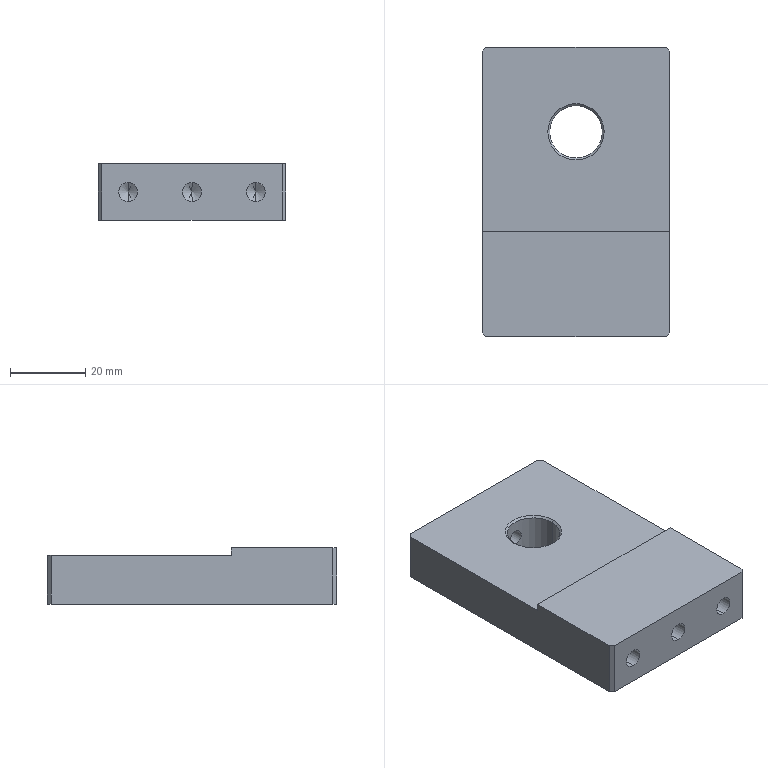Part | NX | features BREP 1 | 1 solid | 40 faces | box 50 x 77 x 15 mm | volume 49360 mm3 | cylinder 14 | cone 14 | plane 12 | commonest cylinder face diameters 5 x6 3.3 x4 4.2 x2 14 x2
STEP:
#1=CARTESIAN_POINT('',(0.,23.,-2.1));
#2=VERTEX_POINT('',#1);
#3=CARTESIAN_POINT('',(0.,23.,2.1));
#4=VERTEX_POINT('',#3);
#5=CARTESIAN_POINT('',(0.,23.,2.1));
#6=CARTESIAN_POINT('',(-0.262,23.,2.1));
#7=CARTESIAN_POINT('',(-0.7456,22.966,1.986));
#8=CARTESIAN_POINT('',(-1.093,22.916,1.805));
#9=CARTESIAN_POINT('',(-1.501,22.841,1.507));
#10=CARTESIAN_POINT('',(-1.817,22.762,1.075));
#11=CARTESIAN_POINT('',(-1.934,22.728,0.8436));
#12=CARTESIAN_POINT('',(-2.082,22.684,0.3873));
#13=CARTESIAN_POINT('',(-2.109,22.674,-0.00003847));
#14=CARTESIAN_POINT('',(-2.082,22.684,-0.3881));
#15=CARTESIAN_POINT('',(-1.934,22.728,-0.844));
#16=CARTESIAN_POINT('',(-1.817,22.762,-1.075));
#17=CARTESIAN_POINT('',(-1.5,22.842,-1.508));
#18=CARTESIAN_POINT('',(-1.092,22.916,-1.805));
#19=CARTESIAN_POINT('',(-0.7431,22.967,-1.987));
#20=CARTESIAN_POINT('',(-0.2615,23.,-2.1));
#21=CARTESIAN_POINT('',(0.,23.,-2.1));
#22=B_SPLINE_CURVE_WITH_KNOTS('',3,(#5,#6,#7,#8,#9,#10,#11,#12,#13,#14,#15,#16,#17,#18,#19,#20,#21),.UNSPECIFIED.,.F.,.F.,(4,1,1,1,1,1,1,1,1,1,1,1,1,1,4),(0.,0.125,0.1875,0.25,0.3125,0.375,0.4375,0.5,0.5625,0.625,0.6875,0.75,0.8125,0.875,1.),.UNSPECIFIED.);
#23=EDGE_CURVE('',#2,#4,#22,.F.);
#24=ORIENTED_EDGE('',*,*,#23,.F.);
#25=CARTESIAN_POINT('',(0.,38.5,-2.1));
#26=VERTEX_POINT('',#25);
#27=CARTESIAN_POINT('',(0.,38.5,-2.1));
#28=DIRECTION('',(0.,1.,0.));
#29=VECTOR('',#28,1000.);
#30=LINE('',#27,#29);
#31=EDGE_CURVE('',#26,#2,#30,.F.);
#32=ORIENTED_EDGE('',*,*,#31,.F.);
#33=CARTESIAN_POINT('',(0.,38.5,2.1));
#34=VERTEX_POINT('',#33);
#35=CARTESIAN_POINT('',(0.,38.5,0.));
#36=DIRECTION('',(0.,1.,0.));
#37=DIRECTION('',(0.,0.,1.));
#38=AXIS2_PLACEMENT_3D('',#35,#36,#37);
#39=CIRCLE('',#38,2.1);
#40=EDGE_CURVE('',#26,#34,#39,.T.);
#41=ORIENTED_EDGE('',*,*,#40,.T.);
#42=CARTESIAN_POINT('',(0.,38.5,2.1));
#43=DIRECTION('',(0.,1.,0.));
#44=VECTOR('',#43,1000.);
#45=LINE('',#42,#44);
#46=EDGE_CURVE('',#34,#4,#45,.F.);
#47=ORIENTED_EDGE('',*,*,#46,.T.);
#48=EDGE_LOOP('',(#24,#32,#41,#47));
#49=FACE_BOUND('',#48,.T.);
#50=CARTESIAN_POINT('',(0.,38.5,0.));
#51=DIRECTION('',(0.,1.,0.));
#52=DIRECTION('',(0.,0.,1.));
#53=AXIS2_PLACEMENT_3D('',#50,#51,#52);
#54=CYLINDRICAL_SURFACE('',#53,2.1);
#55=ADVANCED_FACE('',(#49),#54,.F.);
#56=CARTESIAN_POINT('',(-17.,27.,-1.65));
#57=VERTEX_POINT('',#56);
#58=CARTESIAN_POINT('',(-17.,27.,1.65));
#59=VERTEX_POINT('',#58);
#60=CARTESIAN_POINT('',(-17.,27.,0.));
#61=DIRECTION('',(0.,1.,0.));
#62=DIRECTION('',(0.,0.,1.));
#63=AXIS2_PLACEMENT_3D('',#60,#61,#62);
#64=CIRCLE('',#63,1.65);
#65=EDGE_CURVE('',#57,#59,#64,.T.);
#66=ORIENTED_EDGE('',*,*,#65,.F.);
#67=CARTESIAN_POINT('',(-17.,38.5,-1.65));
#68=VERTEX_POINT('',#67);
#69=CARTESIAN_POINT('',(-17.,38.5,-1.65));
#70=DIRECTION('',(0.,1.,0.));
#71=VECTOR('',#70,1000.);
#72=LINE('',#69,#71);
#73=EDGE_CURVE('',#68,#57,#72,.F.);
#74=ORIENTED_EDGE('',*,*,#73,.F.);
#75=CARTESIAN_POINT('',(-17.,38.5,1.65));
#76=VERTEX_POINT('',#75);
#77=CARTESIAN_POINT('',(-17.,38.5,0.));
#78=DIRECTION('',(0.,1.,0.));
#79=DIRECTION('',(0.,0.,1.));
#80=AXIS2_PLACEMENT_3D('',#77,#78,#79);
#81=CIRCLE('',#80,1.65);
#82=EDGE_CURVE('',#68,#76,#81,.T.);
#83=ORIENTED_EDGE('',*,*,#82,.T.);
#84=CARTESIAN_POINT('',(-17.,38.5,1.65));
#85=DIRECTION('',(0.,1.,0.));
#86=VECTOR('',#85,1000.);
#87=LINE('',#84,#86);
#88=EDGE_CURVE('',#76,#59,#87,.F.);
#89=ORIENTED_EDGE('',*,*,#88,.T.);
#90=EDGE_LOOP('',(#66,#74,#83,#89));
#91=FACE_BOUND('',#90,.T.);
#92=CARTESIAN_POINT('',(-17.,38.5,0.));
#93=DIRECTION('',(0.,1.,0.));
#94=DIRECTION('',(0.,0.,1.));
#95=AXIS2_PLACEMENT_3D('',#92,#93,#94);
#96=CYLINDRICAL_SURFACE('',#95,1.65);
#97=ADVANCED_FACE('',(#91),#96,.F.);
#98=CARTESIAN_POINT('',(-17.,26.009,0.));
#99=VERTEX_POINT('',#98);
#100=CARTESIAN_POINT('',(-17.,27.,1.65));
#101=DIRECTION('',(0.,0.515,0.8572));
#102=VECTOR('',#101,1000.);
#103=LINE('',#100,#102);
#104=EDGE_CURVE('',#59,#99,#103,.F.);
#105=ORIENTED_EDGE('',*,*,#104,.T.);
#106=CARTESIAN_POINT('',(-17.,27.,-1.65));
#107=DIRECTION('',(0.,0.515,-0.8572));
#108=VECTOR('',#107,1000.);
#109=LINE('',#106,#108);
#110=EDGE_CURVE('',#57,#99,#109,.F.);
#111=ORIENTED_EDGE('',*,*,#110,.F.);
#112=ORIENTED_EDGE('',*,*,#65,.T.);
#113=EDGE_LOOP('',(#105,#111,#112));
#114=FACE_BOUND('',#113,.T.);
#115=CARTESIAN_POINT('',(-17.,27.,0.));
#116=DIRECTION('',(0.,1.,0.));
#117=DIRECTION('',(0.,0.,1.));
#118=AXIS2_PLACEMENT_3D('',#115,#116,#117);
#119=CONICAL_SURFACE('',#118,1.65,1.03);
#120=ADVANCED_FACE('',(#114),#119,.F.);
#121=CARTESIAN_POINT('',(17.,27.,-1.65));
#122=VERTEX_POINT('',#121);
#123=CARTESIAN_POINT('',(17.,27.,1.65));
#124=VERTEX_POINT('',#123);
#125=CARTESIAN_POINT('',(17.,27.,0.));
#126=DIRECTION('',(0.,1.,0.));
#127=DIRECTION('',(0.,0.,1.));
#128=AXIS2_PLACEMENT_3D('',#125,#126,#127);
#129=CIRCLE('',#128,1.65);
#130=EDGE_CURVE('',#122,#124,#129,.T.);
#131=ORIENTED_EDGE('',*,*,#130,.F.);
#132=CARTESIAN_POINT('',(17.,38.5,-1.65));
#133=VERTEX_POINT('',#132);
#134=CARTESIAN_POINT('',(17.,38.5,-1.65));
#135=DIRECTION('',(0.,1.,0.));
#136=VECTOR('',#135,1000.);
#137=LINE('',#134,#136);
#138=EDGE_CURVE('',#133,#122,#137,.F.);
#139=ORIENTED_EDGE('',*,*,#138,.F.);
#140=CARTESIAN_POINT('',(17.,38.5,1.65));
#141=VERTEX_POINT('',#140);
#142=CARTESIAN_POINT('',(17.,38.5,0.));
#143=DIRECTION('',(0.,1.,0.));
#144=DIRECTION('',(0.,0.,1.));
#145=AXIS2_PLACEMENT_3D('',#142,#143,#144);
#146=CIRCLE('',#145,1.65);
#147=EDGE_CURVE('',#133,#141,#146,.T.);
#148=ORIENTED_EDGE('',*,*,#147,.T.);
#149=CARTESIAN_POINT('',(17.,38.5,1.65));
#150=DIRECTION('',(0.,1.,0.));
#151=VECTOR('',#150,1000.);
#152=LINE('',#149,#151);
#153=EDGE_CURVE('',#141,#124,#152,.F.);
#154=ORIENTED_EDGE('',*,*,#153,.T.);
#155=EDGE_LOOP('',(#131,#139,#148,#154));
#156=FACE_BOUND('',#155,.T.);
#157=CARTESIAN_POINT('',(17.,38.5,0.));
#158=DIRECTION('',(0.,1.,0.));
#159=DIRECTION('',(0.,0.,1.));
#160=AXIS2_PLACEMENT_3D('',#157,#158,#159);
#161=CYLINDRICAL_SURFACE('',#160,1.65);
#162=ADVANCED_FACE('',(#156),#161,.F.);
#163=CARTESIAN_POINT('',(17.,26.009,0.));
#164=VERTEX_POINT('',#163);
#165=CARTESIAN_POINT('',(17.,27.,1.65));
#166=DIRECTION('',(0.,0.515,0.8572));
#167=VECTOR('',#166,1000.);
#168=LINE('',#165,#167);
#169=EDGE_CURVE('',#124,#164,#168,.F.);
#170=ORIENTED_EDGE('',*,*,#169,.T.);
#171=CARTESIAN_POINT('',(17.,27.,-1.65));
#172=DIRECTION('',(0.,0.515,-0.8572));
#173=VECTOR('',#172,1000.);
#174=LINE('',#171,#173);
#175=EDGE_CURVE('',#122,#164,#174,.F.);
#176=ORIENTED_EDGE('',*,*,#175,.F.);
#177=ORIENTED_EDGE('',*,*,#130,.T.);
#178=EDGE_LOOP('',(#170,#176,#177));
#179=FACE_BOUND('',#178,.T.);
#180=CARTESIAN_POINT('',(17.,27.,0.));
#181=DIRECTION('',(0.,1.,0.));
#182=DIRECTION('',(0.,0.,1.));
#183=AXIS2_PLACEMENT_3D('',#180,#181,#182);
#184=CONICAL_SURFACE('',#183,1.65,1.03);
#185=ADVANCED_FACE('',(#179),#184,.F.);
#186=CARTESIAN_POINT('',(7.,16.,-7.));
#187=VERTEX_POINT('',#186);
#188=CARTESIAN_POINT('',(-7.,16.,-7.));
#189=VERTEX_POINT('',#188);
#190=CARTESIAN_POINT('',(0.,16.,-7.));
#191=DIRECTION('',(0.,0.,-1.));
#192=DIRECTION('',(-1.,0.,0.));
#193=AXIS2_PLACEMENT_3D('',#190,#191,#192);
#194=CIRCLE('',#193,7.);
#195=EDGE_CURVE('',#187,#189,#194,.T.);
#196=ORIENTED_EDGE('',*,*,#195,.F.);
#197=CARTESIAN_POINT('',(7.5,16.,-7.5));
#198=VERTEX_POINT('',#197);
#199=CARTESIAN_POINT('',(7.5,16.,-7.5));
#200=DIRECTION('',(0.7071,0.,-0.7071));
#201=VECTOR('',#200,1000.);
#202=LINE('',#199,#201);
#203=EDGE_CURVE('',#187,#198,#202,.T.);
#204=ORIENTED_EDGE('',*,*,#203,.T.);
#205=CARTESIAN_POINT('',(-7.5,16.,-7.5));
#206=VERTEX_POINT('',#205);
#207=CARTESIAN_POINT('',(0.,16.,-7.5));
#208=DIRECTION('',(0.,0.,1.));
#209=DIRECTION('',(-1.,0.,0.));
#210=AXIS2_PLACEMENT_3D('',#207,#208,#209);
#211=CIRCLE('',#210,7.5);
#212=EDGE_CURVE('',#206,#198,#211,.T.);
#213=ORIENTED_EDGE('',*,*,#212,.F.);
#214=CARTESIAN_POINT('',(-7.5,16.,-7.5));
#215=DIRECTION('',(-0.7071,0.,-0.7071));
#216=VECTOR('',#215,1000.);
#217=LINE('',#214,#216);
#218=EDGE_CURVE('',#189,#206,#217,.T.);
#219=ORIENTED_EDGE('',*,*,#218,.F.);
#220=EDGE_LOOP('',(#196,#204,#213,#219));
#221=FACE_BOUND('',#220,.T.);
#222=CARTESIAN_POINT('',(0.,16.,-7.5));
#223=DIRECTION('',(0.,0.,-1.));
#224=DIRECTION('',(-1.,0.,0.));
#225=AXIS2_PLACEMENT_3D('',#222,#223,#224);
#226=CONICAL_SURFACE('',#225,7.5,0.7854);
#227=ADVANCED_FACE('',(#221),#226,.F.);
#228=CARTESIAN_POINT('',(-7.,16.,5.));
#229=VERTEX_POINT('',#228);
#230=CARTESIAN_POINT('',(7.,16.,5.));
#231=VERTEX_POINT('',#230);
#232=CARTESIAN_POINT('',(0.,16.,5.));
#233=DIRECTION('',(0.,0.,1.));
#234=DIRECTION('',(1.,0.,0.));
#235=AXIS2_PLACEMENT_3D('',#232,#233,#234);
#236=CIRCLE('',#235,7.);
#237=EDGE_CURVE('',#229,#231,#236,.T.);
#238=ORIENTED_EDGE('',*,*,#237,.F.);
#239=CARTESIAN_POINT('',(-7.5,16.,5.5));
#240=VERTEX_POINT('',#239);
#241=CARTESIAN_POINT('',(-7.5,16.,5.5));
#242=DIRECTION('',(-0.7071,0.,0.7071));
#243=VECTOR('',#242,1000.);
#244=LINE('',#241,#243);
#245=EDGE_CURVE('',#240,#229,#244,.F.);
#246=ORIENTED_EDGE('',*,*,#245,.F.);
#247=CARTESIAN_POINT('',(7.5,16.,5.5));
#248=VERTEX_POINT('',#247);
#249=CARTESIAN_POINT('',(0.,16.,5.5));
#250=DIRECTION('',(0.,0.,-1.));
#251=DIRECTION('',(1.,0.,0.));
#252=AXIS2_PLACEMENT_3D('',#249,#250,#251);
#253=CIRCLE('',#252,7.5);
#254=EDGE_CURVE('',#248,#240,#253,.T.);
#255=ORIENTED_EDGE('',*,*,#254,.F.);
#256=CARTESIAN_POINT('',(7.5,16.,5.5));
#257=DIRECTION('',(0.7071,0.,0.7071));
#258=VECTOR('',#257,1000.);
#259=LINE('',#256,#258);
#260=EDGE_CURVE('',#248,#231,#259,.F.);
#261=ORIENTED_EDGE('',*,*,#260,.T.);
#262=EDGE_LOOP('',(#238,#246,#255,#261));
#263=FACE_BOUND('',#262,.T.);
#264=CARTESIAN_POINT('',(0.,16.,5.5));
#265=DIRECTION('',(0.,0.,1.));
#266=DIRECTION('',(1.,0.,0.));
#267=AXIS2_PLACEMENT_3D('',#264,#265,#266);
#268=CONICAL_SURFACE('',#267,7.5,0.7854);
#269=ADVANCED_FACE('',(#263),#268,.F.);
#270=CARTESIAN_POINT('',(-17.,-21.5,2.5));
#271=VERTEX_POINT('',#270);
#272=CARTESIAN_POINT('',(-17.,-21.5,-2.5));
#273=VERTEX_POINT('',#272);
#274=CARTESIAN_POINT('',(-17.,-21.5,0.));
#275=DIRECTION('',(0.,-1.,0.));
#276=DIRECTION('',(0.,0.,-1.));
#277=AXIS2_PLACEMENT_3D('',#274,#275,#276);
#278=CIRCLE('',#277,2.5);
#279=EDGE_CURVE('',#271,#273,#278,.T.);
#280=ORIENTED_EDGE('',*,*,#279,.F.);
#281=CARTESIAN_POINT('',(-17.,-38.5,2.5));
#282=VERTEX_POINT('',#281);
#283=CARTESIAN_POINT('',(-17.,-38.5,2.5));
#284=DIRECTION('',(0.,-1.,0.));
#285=VECTOR('',#284,1000.);
#286=LINE('',#283,#285);
#287=EDGE_CURVE('',#271,#282,#286,.T.);
#288=ORIENTED_EDGE('',*,*,#287,.T.);
#289=CARTESIAN_POINT('',(-17.,-38.5,-2.5));
#290=VERTEX_POINT('',#289);
#291=CARTESIAN_POINT('',(-17.,-38.5,0.));
#292=DIRECTION('',(0.,-1.,0.));
#293=DIRECTION('',(0.,0.,-1.));
#294=AXIS2_PLACEMENT_3D('',#291,#292,#293);
#295=CIRCLE('',#294,2.5);
#296=EDGE_CURVE('',#282,#290,#295,.T.);
#297=ORIENTED_EDGE('',*,*,#296,.T.);
#298=CARTESIAN_POINT('',(-17.,-38.5,-2.5));
#299=DIRECTION('',(0.,-1.,0.));
#300=VECTOR('',#299,1000.);
#301=LINE('',#298,#300);
#302=EDGE_CURVE('',#273,#290,#301,.T.);
#303=ORIENTED_EDGE('',*,*,#302,.F.);
#304=EDGE_LOOP('',(#280,#288,#297,#303));
#305=FACE_BOUND('',#304,.T.);
#306=CARTESIAN_POINT('',(-17.,-38.5,0.));
#307=DIRECTION('',(0.,-1.,0.));
#308=DIRECTION('',(0.,0.,-1.));
#309=AXIS2_PLACEMENT_3D('',#306,#307,#308);
#310=CYLINDRICAL_SURFACE('',#309,2.5);
#311=ADVANCED_FACE('',(#305),#310,.F.);
#312=CARTESIAN_POINT('',(-17.,-19.998,0.));
#313=VERTEX_POINT('',#312);
#314=CARTESIAN_POINT('',(-17.,-21.5,-2.5));
#315=DIRECTION('',(0.,-0.515,-0.8572));
#316=VECTOR('',#315,1000.);
#317=LINE('',#314,#316);
#318=EDGE_CURVE('',#313,#273,#317,.T.);
#319=ORIENTED_EDGE('',*,*,#318,.F.);
#320=CARTESIAN_POINT('',(-17.,-21.5,2.5));
#321=DIRECTION('',(0.,-0.515,0.8572));
#322=VECTOR('',#321,1000.);
#323=LINE('',#320,#322);
#324=EDGE_CURVE('',#313,#271,#323,.T.);
#325=ORIENTED_EDGE('',*,*,#324,.T.);
#326=ORIENTED_EDGE('',*,*,#279,.T.);
#327=EDGE_LOOP('',(#319,#325,#326));
#328=FACE_BOUND('',#327,.T.);
#329=CARTESIAN_POINT('',(-17.,-21.5,0.));
#330=DIRECTION('',(0.,-1.,0.));
#331=DIRECTION('',(0.,0.,-1.));
#332=AXIS2_PLACEMENT_3D('',#329,#330,#331);
#333=CONICAL_SURFACE('',#332,2.5,1.03);
#334=ADVANCED_FACE('',(#328),#333,.F.);
#335=CARTESIAN_POINT('',(0.,-21.5,2.5));
#336=VERTEX_POINT('',#335);
#337=CARTESIAN_POINT('',(0.,-21.5,-2.5));
#338=VERTEX_POINT('',#337);
#339=CARTESIAN_POINT('',(0.,-21.5,0.));
#340=DIRECTION('',(0.,-1.,0.));
#341=DIRECTION('',(0.,0.,-1.));
#342=AXIS2_PLACEMENT_3D('',#339,#340,#341);
#343=CIRCLE('',#342,2.5);
#344=EDGE_CURVE('',#336,#338,#343,.T.);
#345=ORIENTED_EDGE('',*,*,#344,.F.);
#346=CARTESIAN_POINT('',(0.,-38.5,2.5));
#347=VERTEX_POINT('',#346);
#348=CARTESIAN_POINT('',(0.,-38.5,2.5));
#349=DIRECTION('',(0.,-1.,0.));
#350=VECTOR('',#349,1000.);
#351=LINE('',#348,#350);
#352=EDGE_CURVE('',#336,#347,#351,.T.);
#353=ORIENTED_EDGE('',*,*,#352,.T.);
#354=CARTESIAN_POINT('',(0.,-38.5,-2.5));
#355=VERTEX_POINT('',#354);
#356=CARTESIAN_POINT('',(0.,-38.5,0.));
#357=DIRECTION('',(0.,-1.,0.));
#358=DIRECTION('',(0.,0.,-1.));
#359=AXIS2_PLACEMENT_3D('',#356,#357,#358);
#360=CIRCLE('',#359,2.5);
#361=EDGE_CURVE('',#347,#355,#360,.T.);
#362=ORIENTED_EDGE('',*,*,#361,.T.);
#363=CARTESIAN_POINT('',(0.,-38.5,-2.5));
#364=DIRECTION('',(0.,-1.,0.));
#365=VECTOR('',#364,1000.);
#366=LINE('',#363,#365);
#367=EDGE_CURVE('',#338,#355,#366,.T.);
#368=ORIENTED_EDGE('',*,*,#367,.F.);
#369=EDGE_LOOP('',(#345,#353,#362,#368));
#370=FACE_BOUND('',#369,.T.);
#371=CARTESIAN_POINT('',(0.,-38.5,0.));
#372=DIRECTION('',(0.,-1.,0.));
#373=DIRECTION('',(0.,0.,-1.));
#374=AXIS2_PLACEMENT_3D('',#371,#372,#373);
#375=CYLINDRICAL_SURFACE('',#374,2.5);
#376=ADVANCED_FACE('',(#370),#375,.F.);
#377=CARTESIAN_POINT('',(0.,-19.998,0.));
#378=VERTEX_POINT('',#377);
#379=CARTESIAN_POINT('',(0.,-21.5,-2.5));
#380=DIRECTION('',(0.,-0.515,-0.8572));
#381=VECTOR('',#380,1000.);
#382=LINE('',#379,#381);
#383=EDGE_CURVE('',#378,#338,#382,.T.);
#384=ORIENTED_EDGE('',*,*,#383,.F.);
#385=CARTESIAN_POINT('',(0.,-21.5,2.5));
#386=DIRECTION('',(0.,-0.515,0.8572));
#387=VECTOR('',#386,1000.);
#388=LINE('',#385,#387);
#389=EDGE_CURVE('',#378,#336,#388,.T.);
#390=ORIENTED_EDGE('',*,*,#389,.T.);
#391=ORIENTED_EDGE('',*,*,#344,.T.);
#392=EDGE_LOOP('',(#384,#390,#391));
#393=FACE_BOUND('',#392,.T.);
#394=CARTESIAN_POINT('',(0.,-21.5,0.));
#395=DIRECTION('',(0.,-1.,0.));
#396=DIRECTION('',(0.,0.,-1.));
#397=AXIS2_PLACEMENT_3D('',#394,#395,#396);
#398=CONICAL_SURFACE('',#397,2.5,1.03);
#399=ADVANCED_FACE('',(#393),#398,.F.);
#400=CARTESIAN_POINT('',(17.,-21.5,2.5));
#401=VERTEX_POINT('',#400);
#402=CARTESIAN_POINT('',(17.,-21.5,-2.5));
#403=VERTEX_POINT('',#402);
#404=CARTESIAN_POINT('',(17.,-21.5,0.));
#405=DIRECTION('',(0.,-1.,0.));
#406=DIRECTION('',(0.,0.,-1.));
#407=AXIS2_PLACEMENT_3D('',#404,#405,#406);
#408=CIRCLE('',#407,2.5);
#409=EDGE_CURVE('',#401,#403,#408,.T.);
#410=ORIENTED_EDGE('',*,*,#409,.F.);
#411=CARTESIAN_POINT('',(17.,-38.5,2.5));
#412=VERTEX_POINT('',#411);
#413=CARTESIAN_POINT('',(17.,-38.5,2.5));
#414=DIRECTION('',(0.,-1.,0.));
#415=VECTOR('',#414,1000.);
#416=LINE('',#413,#415);
#417=EDGE_CURVE('',#401,#412,#416,.T.);
#418=ORIENTED_EDGE('',*,*,#417,.T.);
#419=CARTESIAN_POINT('',(17.,-38.5,-2.5));
#420=VERTEX_POINT('',#419);
#421=CARTESIAN_POINT('',(17.,-38.5,0.));
#422=DIRECTION('',(0.,-1.,0.));
#423=DIRECTION('',(0.,0.,-1.));
#424=AXIS2_PLACEMENT_3D('',#421,#422,#423);
#425=CIRCLE('',#424,2.5);
#426=EDGE_CURVE('',#412,#420,#425,.T.);
#427=ORIENTED_EDGE('',*,*,#426,.T.);
#428=CARTESIAN_POINT('',(17.,-38.5,-2.5));
#429=DIRECTION('',(0.,-1.,0.));
#430=VECTOR('',#429,1000.);
#431=LINE('',#428,#430);
#432=EDGE_CURVE('',#403,#420,#431,.T.);
#433=ORIENTED_EDGE('',*,*,#432,.F.);
#434=EDGE_LOOP('',(#410,#418,#427,#433));
#435=FACE_BOUND('',#434,.T.);
#436=CARTESIAN_POINT('',(17.,-38.5,0.));
#437=DIRECTION('',(0.,-1.,0.));
#438=DIRECTION('',(0.,0.,-1.));
#439=AXIS2_PLACEMENT_3D('',#436,#437,#438);
#440=CYLINDRICAL_SURFACE('',#439,2.5);
#441=ADVANCED_FACE('',(#435),#440,.F.);
#442=CARTESIAN_POINT('',(17.,-19.998,0.));
#443=VERTEX_POINT('',#442);
#444=CARTESIAN_POINT('',(17.,-21.5,-2.5));
#445=DIRECTION('',(0.,-0.515,-0.8572));
#446=VECTOR('',#445,1000.);
#447=LINE('',#444,#446);
#448=EDGE_CURVE('',#443,#403,#447,.T.);
#449=ORIENTED_EDGE('',*,*,#448,.F.);
#450=CARTESIAN_POINT('',(17.,-21.5,2.5));
#451=DIRECTION('',(0.,-0.515,0.8572));
#452=VECTOR('',#451,1000.);
#453=LINE('',#450,#452);
#454=EDGE_CURVE('',#443,#401,#453,.T.);
#455=ORIENTED_EDGE('',*,*,#454,.T.);
#456=ORIENTED_EDGE('',*,*,#409,.T.);
#457=EDGE_LOOP('',(#449,#455,#456));
#458=FACE_BOUND('',#457,.T.);
#459=CARTESIAN_POINT('',(17.,-21.5,0.));
#460=DIRECTION('',(0.,-1.,0.));
#461=DIRECTION('',(0.,0.,-1.));
#462=AXIS2_PLACEMENT_3D('',#459,#460,#461);
#463=CONICAL_SURFACE('',#462,2.5,1.03);
#464=ADVANCED_FACE('',(#458),#463,.F.);
#465=ORIENTED_EDGE('',*,*,#195,.T.);
#466=CARTESIAN_POINT('',(-7.,16.,-7.5));
#467=DIRECTION('',(0.,0.,1.));
#468=VECTOR('',#467,1000.);
#469=LINE('',#466,#468);
#470=EDGE_CURVE('',#229,#189,#469,.F.);
#471=ORIENTED_EDGE('',*,*,#470,.F.);
#472=ORIENTED_EDGE('',*,*,#237,.T.);
#473=CARTESIAN_POINT('',(7.,16.,-7.5));
#474=DIRECTION('',(0.,0.,1.));
#475=VECTOR('',#474,1000.);
#476=LINE('',#473,#475);
#477=EDGE_CURVE('',#231,#187,#476,.F.);
#478=ORIENTED_EDGE('',*,*,#477,.T.);
#479=EDGE_LOOP('',(#465,#471,#472,#478));
#480=FACE_BOUND('',#479,.T.);
#481=CARTESIAN_POINT('',(0.,16.,-7.5));
#482=DIRECTION('',(0.,0.,1.));
#483=DIRECTION('',(1.,0.,0.));
#484=AXIS2_PLACEMENT_3D('',#481,#482,#483);
#485=CYLINDRICAL_SURFACE('',#484,7.);
#486=ADVANCED_FACE('',(#480),#485,.F.);
#487=CARTESIAN_POINT('',(24.,38.5,5.5));
#488=VERTEX_POINT('',#487);
#489=CARTESIAN_POINT('',(-24.,38.5,5.5));
#490=VERTEX_POINT('',#489);
#491=CARTESIAN_POINT('',(-25.,38.5,5.5));
#492=DIRECTION('',(-1.,0.,0.));
#493=VECTOR('',#492,1000.);
#494=LINE('',#491,#493);
#495=EDGE_CURVE('',#488,#490,#494,.T.);
#496=ORIENTED_EDGE('',*,*,#495,.F.);
#497=CARTESIAN_POINT('',(24.,38.5,-7.5));
#498=VERTEX_POINT('',#497);
#499=CARTESIAN_POINT('',(24.,38.5,7.5));
#500=DIRECTION('',(0.,0.,-1.));
#501=VECTOR('',#500,1000.);
#502=LINE('',#499,#501);
#503=EDGE_CURVE('',#488,#498,#502,.T.);
#504=ORIENTED_EDGE('',*,*,#503,.T.);
#505=CARTESIAN_POINT('',(-24.,38.5,-7.5));
#506=VERTEX_POINT('',#505);
#507=CARTESIAN_POINT('',(-25.,38.5,-7.5));
#508=DIRECTION('',(-1.,0.,0.));
#509=VECTOR('',#508,1000.);
#510=LINE('',#507,#509);
#511=EDGE_CURVE('',#498,#506,#510,.T.);
#512=ORIENTED_EDGE('',*,*,#511,.T.);
#513=CARTESIAN_POINT('',(-24.,38.5,7.5));
#514=DIRECTION('',(0.,0.,1.));
#515=VECTOR('',#514,1000.);
#516=LINE('',#513,#515);
#517=EDGE_CURVE('',#506,#490,#516,.T.);
#518=ORIENTED_EDGE('',*,*,#517,.T.);
#519=EDGE_LOOP('',(#496,#504,#512,#518));
#520=FACE_BOUND('',#519,.T.);
#521=CARTESIAN_POINT('',(17.,38.5,0.));
#522=DIRECTION('',(0.,1.,0.));
#523=DIRECTION('',(0.,0.,1.));
#524=AXIS2_PLACEMENT_3D('',#521,#522,#523);
#525=CIRCLE('',#524,1.65);
#526=EDGE_CURVE('',#141,#133,#525,.T.);
#527=ORIENTED_EDGE('',*,*,#526,.F.);
#528=ORIENTED_EDGE('',*,*,#147,.F.);
#529=EDGE_LOOP('',(#527,#528));
#530=FACE_BOUND('',#529,.T.);
#531=CARTESIAN_POINT('',(-17.,38.5,0.));
#532=DIRECTION('',(0.,1.,0.));
#533=DIRECTION('',(0.,0.,1.));
#534=AXIS2_PLACEMENT_3D('',#531,#532,#533);
#535=CIRCLE('',#534,1.65);
#536=EDGE_CURVE('',#76,#68,#535,.T.);
#537=ORIENTED_EDGE('',*,*,#536,.F.);
#538=ORIENTED_EDGE('',*,*,#82,.F.);
#539=EDGE_LOOP('',(#537,#538));
#540=FACE_BOUND('',#539,.T.);
#541=CARTESIAN_POINT('',(0.,38.5,0.));
#542=DIRECTION('',(0.,1.,0.));
#543=DIRECTION('',(0.,0.,1.));
#544=AXIS2_PLACEMENT_3D('',#541,#542,#543);
#545=CIRCLE('',#544,2.1);
#546=EDGE_CURVE('',#34,#26,#545,.T.);
#547=ORIENTED_EDGE('',*,*,#546,.F.);
#548=ORIENTED_EDGE('',*,*,#40,.F.);
#549=EDGE_LOOP('',(#547,#548));
#550=FACE_BOUND('',#549,.T.);
#551=CARTESIAN_POINT('',(-25.,38.5,7.5));
#552=DIRECTION('',(0.,-1.,0.));
#553=DIRECTION('',(0.,0.,-1.));
#554=AXIS2_PLACEMENT_3D('',#551,#552,#553);
#555=PLANE('',#554);
#556=ADVANCED_FACE('',(#520,#530,#540,#550),#555,.F.);
#557=ORIENTED_EDGE('',*,*,#470,.T.);
#558=CARTESIAN_POINT('',(0.,16.,-7.));
#559=DIRECTION('',(0.,0.,-1.));
#560=DIRECTION('',(-1.,0.,0.));
#561=AXIS2_PLACEMENT_3D('',#558,#559,#560);
#562=CIRCLE('',#561,7.);
#563=EDGE_CURVE('',#189,#187,#562,.T.);
#564=ORIENTED_EDGE('',*,*,#563,.T.);
#565=ORIENTED_EDGE('',*,*,#477,.F.);
#566=CARTESIAN_POINT('',(0.,16.,5.));
#567=DIRECTION('',(0.,0.,1.));
#568=DIRECTION('',(1.,0.,0.));
#569=AXIS2_PLACEMENT_3D('',#566,#567,#568);
#570=CIRCLE('',#569,7.);
#571=EDGE_CURVE('',#231,#229,#570,.T.);
#572=ORIENTED_EDGE('',*,*,#571,.T.);
#573=EDGE_LOOP('',(#557,#564,#565,#572));
#574=FACE_BOUND('',#573,.T.);
#575=CARTESIAN_POINT('',(0.,23.,2.1));
#576=CARTESIAN_POINT('',(0.5584,23.,2.1));
#577=CARTESIAN_POINT('',(1.642,22.842,1.644));
#578=CARTESIAN_POINT('',(2.33,22.595,0.002212));
#579=CARTESIAN_POINT('',(1.64,22.843,-1.647));
#580=CARTESIAN_POINT('',(0.5576,23.,-2.1));
#581=CARTESIAN_POINT('',(0.,23.,-2.1));
#582=B_SPLINE_CURVE_WITH_KNOTS('',3,(#575,#576,#577,#578,#579,#580,#581),.UNSPECIFIED.,.F.,.F.,(4,1,1,1,4),(0.,0.25,0.5,0.75,1.),.UNSPECIFIED.);
#583=EDGE_CURVE('',#4,#2,#582,.T.);
#584=ORIENTED_EDGE('',*,*,#583,.T.);
#585=ORIENTED_EDGE('',*,*,#23,.T.);
#586=EDGE_LOOP('',(#584,#585));
#587=FACE_BOUND('',#586,.T.);
#588=CARTESIAN_POINT('',(0.,16.,-7.5));
#589=DIRECTION('',(0.,0.,1.));
#590=DIRECTION('',(1.,0.,0.));
#591=AXIS2_PLACEMENT_3D('',#588,#589,#590);
#592=CYLINDRICAL_SURFACE('',#591,7.);
#593=ADVANCED_FACE('',(#574,#587),#592,.F.);
#594=ORIENTED_EDGE('',*,*,#503,.F.);
#595=CARTESIAN_POINT('',(25.,37.5,5.5));
#596=VERTEX_POINT('',#595);
#597=CARTESIAN_POINT('',(24.,38.5,5.5));
#598=DIRECTION('',(0.7071,-0.7071,0.));
#599=VECTOR('',#598,1000.);
#600=LINE('',#597,#599);
#601=EDGE_CURVE('',#488,#596,#600,.T.);
#602=ORIENTED_EDGE('',*,*,#601,.T.);
#603=CARTESIAN_POINT('',(25.,37.5,-7.5));
#604=VERTEX_POINT('',#603);
#605=CARTESIAN_POINT('',(25.,37.5,7.5));
#606=DIRECTION('',(0.,0.,1.));
#607=VECTOR('',#606,1000.);
#608=LINE('',#605,#607);
#609=EDGE_CURVE('',#604,#596,#608,.T.);
#610=ORIENTED_EDGE('',*,*,#609,.F.);
#611=CARTESIAN_POINT('',(31.25,31.25,-7.5));
#612=DIRECTION('',(0.7071,-0.7071,0.));
#613=VECTOR('',#612,1000.);
#614=LINE('',#611,#613);
#615=EDGE_CURVE('',#498,#604,#614,.T.);
#616=ORIENTED_EDGE('',*,*,#615,.F.);
#617=EDGE_LOOP('',(#594,#602,#610,#616));
#618=FACE_BOUND('',#617,.T.);
#619=CARTESIAN_POINT('',(24.,38.5,7.5));
#620=DIRECTION('',(-0.7071,-0.7071,0.));
#621=DIRECTION('',(-0.7071,0.7071,0.));
#622=AXIS2_PLACEMENT_3D('',#619,#620,#621);
#623=PLANE('',#622);
#624=ADVANCED_FACE('',(#618),#623,.F.);
#625=CARTESIAN_POINT('',(-25.,37.5,5.5));
#626=VERTEX_POINT('',#625);
#627=CARTESIAN_POINT('',(-25.,37.5,-7.5));
#628=VERTEX_POINT('',#627);
#629=CARTESIAN_POINT('',(-25.,37.5,7.5));
#630=DIRECTION('',(0.,0.,-1.));
#631=VECTOR('',#630,1000.);
#632=LINE('',#629,#631);
#633=EDGE_CURVE('',#626,#628,#632,.T.);
#634=ORIENTED_EDGE('',*,*,#633,.F.);
#635=CARTESIAN_POINT('',(-25.,37.5,5.5));
#636=DIRECTION('',(0.7071,0.7071,0.));
#637=VECTOR('',#636,1000.);
#638=LINE('',#635,#637);
#639=EDGE_CURVE('',#626,#490,#638,.T.);
#640=ORIENTED_EDGE('',*,*,#639,.T.);
#641=ORIENTED_EDGE('',*,*,#517,.F.);
#642=CARTESIAN_POINT('',(-31.25,31.25,-7.5));
#643=DIRECTION('',(0.7071,0.7071,0.));
#644=VECTOR('',#643,1000.);
#645=LINE('',#642,#644);
#646=EDGE_CURVE('',#628,#506,#645,.T.);
#647=ORIENTED_EDGE('',*,*,#646,.F.);
#648=EDGE_LOOP('',(#634,#640,#641,#647));
#649=FACE_BOUND('',#648,.T.);
#650=CARTESIAN_POINT('',(-25.,37.5,7.5));
#651=DIRECTION('',(0.7071,-0.7071,0.));
#652=DIRECTION('',(0.,0.,-1.));
#653=AXIS2_PLACEMENT_3D('',#650,#651,#652);
#654=PLANE('',#653);
#655=ADVANCED_FACE('',(#649),#654,.F.);
#656=CARTESIAN_POINT('',(-24.,-38.5,7.5));
#657=VERTEX_POINT('',#656);
#658=CARTESIAN_POINT('',(24.,-38.5,7.5));
#659=VERTEX_POINT('',#658);
#660=CARTESIAN_POINT('',(-25.,-38.5,7.5));
#661=DIRECTION('',(1.,0.,0.));
#662=VECTOR('',#661,1000.);
#663=LINE('',#660,#662);
#664=EDGE_CURVE('',#657,#659,#663,.T.);
#665=ORIENTED_EDGE('',*,*,#664,.F.);
#666=CARTESIAN_POINT('',(-24.,-38.5,-7.5));
#667=VERTEX_POINT('',#666);
#668=CARTESIAN_POINT('',(-24.,-38.5,7.5));
#669=DIRECTION('',(0.,0.,-1.));
#670=VECTOR('',#669,1000.);
#671=LINE('',#668,#670);
#672=EDGE_CURVE('',#657,#667,#671,.T.);
#673=ORIENTED_EDGE('',*,*,#672,.T.);
#674=CARTESIAN_POINT('',(24.,-38.5,-7.5));
#675=VERTEX_POINT('',#674);
#676=CARTESIAN_POINT('',(-25.,-38.5,-7.5));
#677=DIRECTION('',(1.,0.,0.));
#678=VECTOR('',#677,1000.);
#679=LINE('',#676,#678);
#680=EDGE_CURVE('',#667,#675,#679,.T.);
#681=ORIENTED_EDGE('',*,*,#680,.T.);
#682=CARTESIAN_POINT('',(24.,-38.5,7.5));
#683=DIRECTION('',(0.,0.,1.));
#684=VECTOR('',#683,1000.);
#685=LINE('',#682,#684);
#686=EDGE_CURVE('',#675,#659,#685,.T.);
#687=ORIENTED_EDGE('',*,*,#686,.T.);
#688=EDGE_LOOP('',(#665,#673,#681,#687));
#689=FACE_BOUND('',#688,.T.);
#690=CARTESIAN_POINT('',(17.,-38.5,0.));
#691=DIRECTION('',(0.,-1.,0.));
#692=DIRECTION('',(0.,0.,-1.));
#693=AXIS2_PLACEMENT_3D('',#690,#691,#692);
#694=CIRCLE('',#693,2.5);
#695=EDGE_CURVE('',#420,#412,#694,.T.);
#696=ORIENTED_EDGE('',*,*,#695,.F.);
#697=ORIENTED_EDGE('',*,*,#426,.F.);
#698=EDGE_LOOP('',(#696,#697));
#699=FACE_BOUND('',#698,.T.);
#700=CARTESIAN_POINT('',(0.,-38.5,0.));
#701=DIRECTION('',(0.,-1.,0.));
#702=DIRECTION('',(0.,0.,-1.));
#703=AXIS2_PLACEMENT_3D('',#700,#701,#702);
#704=CIRCLE('',#703,2.5);
#705=EDGE_CURVE('',#355,#347,#704,.T.);
#706=ORIENTED_EDGE('',*,*,#705,.F.);
#707=ORIENTED_EDGE('',*,*,#361,.F.);
#708=EDGE_LOOP('',(#706,#707));
#709=FACE_BOUND('',#708,.T.);
#710=CARTESIAN_POINT('',(-17.,-38.5,0.));
#711=DIRECTION('',(0.,-1.,0.));
#712=DIRECTION('',(0.,0.,-1.));
#713=AXIS2_PLACEMENT_3D('',#710,#711,#712);
#714=CIRCLE('',#713,2.5);
#715=EDGE_CURVE('',#290,#282,#714,.T.);
#716=ORIENTED_EDGE('',*,*,#715,.F.);
#717=ORIENTED_EDGE('',*,*,#296,.F.);
#718=EDGE_LOOP('',(#716,#717));
#719=FACE_BOUND('',#718,.T.);
#720=CARTESIAN_POINT('',(-25.,-38.5,7.5));
#721=DIRECTION('',(0.,1.,0.));
#722=DIRECTION('',(1.,0.,0.));
#723=AXIS2_PLACEMENT_3D('',#720,#721,#722);
#724=PLANE('',#723);
#725=ADVANCED_FACE('',(#689,#699,#709,#719),#724,.F.);
#726=CARTESIAN_POINT('',(25.,-10.5,5.5));
#727=VERTEX_POINT('',#726);
#728=CARTESIAN_POINT('',(25.,-38.5,5.5));
#729=DIRECTION('',(0.,1.,0.));
#730=VECTOR('',#729,1000.);
#731=LINE('',#728,#730);
#732=EDGE_CURVE('',#727,#596,#731,.T.);
#733=ORIENTED_EDGE('',*,*,#732,.F.);
#734=CARTESIAN_POINT('',(25.,-10.5,7.5));
#735=VERTEX_POINT('',#734);
#736=CARTESIAN_POINT('',(25.,-10.5,7.5));
#737=DIRECTION('',(0.,0.,1.));
#738=VECTOR('',#737,1000.);
#739=LINE('',#736,#738);
#740=EDGE_CURVE('',#727,#735,#739,.T.);
#741=ORIENTED_EDGE('',*,*,#740,.T.);
#742=CARTESIAN_POINT('',(25.,-37.5,7.5));
#743=VERTEX_POINT('',#742);
#744=CARTESIAN_POINT('',(25.,-38.5,7.5));
#745=DIRECTION('',(0.,1.,0.));
#746=VECTOR('',#745,1000.);
#747=LINE('',#744,#746);
#748=EDGE_CURVE('',#743,#735,#747,.T.);
#749=ORIENTED_EDGE('',*,*,#748,.F.);
#750=CARTESIAN_POINT('',(25.,-37.5,-7.5));
#751=VERTEX_POINT('',#750);
#752=CARTESIAN_POINT('',(25.,-37.5,7.5));
#753=DIRECTION('',(0.,0.,-1.));
#754=VECTOR('',#753,1000.);
#755=LINE('',#752,#754);
#756=EDGE_CURVE('',#743,#751,#755,.T.);
#757=ORIENTED_EDGE('',*,*,#756,.T.);
#758=CARTESIAN_POINT('',(25.,-38.5,-7.5));
#759=DIRECTION('',(0.,1.,0.));
#760=VECTOR('',#759,1000.);
#761=LINE('',#758,#760);
#762=EDGE_CURVE('',#751,#604,#761,.T.);
#763=ORIENTED_EDGE('',*,*,#762,.T.);
#764=ORIENTED_EDGE('',*,*,#609,.T.);
#765=EDGE_LOOP('',(#733,#741,#749,#757,#763,#764));
#766=FACE_BOUND('',#765,.T.);
#767=CARTESIAN_POINT('',(25.,-38.5,7.5));
#768=DIRECTION('',(-1.,0.,0.));
#769=DIRECTION('',(0.,0.,1.));
#770=AXIS2_PLACEMENT_3D('',#767,#768,#769);
#771=PLANE('',#770);
#772=ADVANCED_FACE('',(#766),#771,.F.);
#773=CARTESIAN_POINT('',(-25.,-10.5,7.5));
#774=VERTEX_POINT('',#773);
#775=CARTESIAN_POINT('',(-25.,-37.5,7.5));
#776=VERTEX_POINT('',#775);
#777=CARTESIAN_POINT('',(-25.,-38.5,7.5));
#778=DIRECTION('',(0.,-1.,0.));
#779=VECTOR('',#778,1000.);
#780=LINE('',#777,#779);
#781=EDGE_CURVE('',#774,#776,#780,.T.);
#782=ORIENTED_EDGE('',*,*,#781,.F.);
#783=CARTESIAN_POINT('',(-25.,-10.5,5.5));
#784=VERTEX_POINT('',#783);
#785=CARTESIAN_POINT('',(-25.,-10.5,7.5));
#786=DIRECTION('',(0.,0.,-1.));
#787=VECTOR('',#786,1000.);
#788=LINE('',#785,#787);
#789=EDGE_CURVE('',#774,#784,#788,.T.);
#790=ORIENTED_EDGE('',*,*,#789,.T.);
#791=CARTESIAN_POINT('',(-25.,-38.5,5.5));
#792=DIRECTION('',(0.,-1.,0.));
#793=VECTOR('',#792,1000.);
#794=LINE('',#791,#793);
#795=EDGE_CURVE('',#626,#784,#794,.T.);
#796=ORIENTED_EDGE('',*,*,#795,.F.);
#797=ORIENTED_EDGE('',*,*,#633,.T.);
#798=CARTESIAN_POINT('',(-25.,-37.5,-7.5));
#799=VERTEX_POINT('',#798);
#800=CARTESIAN_POINT('',(-25.,-38.5,-7.5));
#801=DIRECTION('',(0.,-1.,0.));
#802=VECTOR('',#801,1000.);
#803=LINE('',#800,#802);
#804=EDGE_CURVE('',#628,#799,#803,.T.);
#805=ORIENTED_EDGE('',*,*,#804,.T.);
#806=CARTESIAN_POINT('',(-25.,-37.5,7.5));
#807=DIRECTION('',(0.,0.,1.));
#808=VECTOR('',#807,1000.);
#809=LINE('',#806,#808);
#810=EDGE_CURVE('',#799,#776,#809,.T.);
#811=ORIENTED_EDGE('',*,*,#810,.T.);
#812=EDGE_LOOP('',(#782,#790,#796,#797,#805,#811));
#813=FACE_BOUND('',#812,.T.);
#814=CARTESIAN_POINT('',(-25.,-38.5,7.5));
#815=DIRECTION('',(1.,0.,0.));
#816=DIRECTION('',(0.,1.,0.));
#817=AXIS2_PLACEMENT_3D('',#814,#815,#816);
#818=PLANE('',#817);
#819=ADVANCED_FACE('',(#813),#818,.F.);
#820=ORIENTED_EDGE('',*,*,#748,.T.);
#821=CARTESIAN_POINT('',(-34.51,-10.5,7.5));
#822=DIRECTION('',(1.,0.,0.));
#823=VECTOR('',#822,1000.);
#824=LINE('',#821,#823);
#825=EDGE_CURVE('',#774,#735,#824,.T.);
#826=ORIENTED_EDGE('',*,*,#825,.F.);
#827=ORIENTED_EDGE('',*,*,#781,.T.);
#828=CARTESIAN_POINT('',(-24.,-38.5,7.5));
#829=DIRECTION('',(0.7071,-0.7071,0.));
#830=VECTOR('',#829,1000.);
#831=LINE('',#828,#830);
#832=EDGE_CURVE('',#776,#657,#831,.T.);
#833=ORIENTED_EDGE('',*,*,#832,.T.);
#834=ORIENTED_EDGE('',*,*,#664,.T.);
#835=CARTESIAN_POINT('',(25.,-37.5,7.5));
#836=DIRECTION('',(0.7071,0.7071,0.));
#837=VECTOR('',#836,1000.);
#838=LINE('',#835,#837);
#839=EDGE_CURVE('',#659,#743,#838,.T.);
#840=ORIENTED_EDGE('',*,*,#839,.T.);
#841=EDGE_LOOP('',(#820,#826,#827,#833,#834,#840));
#842=FACE_BOUND('',#841,.T.);
#843=CARTESIAN_POINT('',(0.,0.,7.5));
#844=DIRECTION('',(0.,0.,-1.));
#845=DIRECTION('',(0.,-1.,0.));
#846=AXIS2_PLACEMENT_3D('',#843,#844,#845);
#847=PLANE('',#846);
#848=ADVANCED_FACE('',(#842),#847,.F.);
#849=ORIENTED_EDGE('',*,*,#680,.F.);
#850=CARTESIAN_POINT('',(-31.25,-31.25,-7.5));
#851=DIRECTION('',(-0.7071,0.7071,0.));
#852=VECTOR('',#851,1000.);
#853=LINE('',#850,#852);
#854=EDGE_CURVE('',#667,#799,#853,.T.);
#855=ORIENTED_EDGE('',*,*,#854,.T.);
#856=ORIENTED_EDGE('',*,*,#804,.F.);
#857=ORIENTED_EDGE('',*,*,#646,.T.);
#858=ORIENTED_EDGE('',*,*,#511,.F.);
#859=ORIENTED_EDGE('',*,*,#615,.T.);
#860=ORIENTED_EDGE('',*,*,#762,.F.);
#861=CARTESIAN_POINT('',(31.25,-31.25,-7.5));
#862=DIRECTION('',(-0.7071,-0.7071,0.));
#863=VECTOR('',#862,1000.);
#864=LINE('',#861,#863);
#865=EDGE_CURVE('',#751,#675,#864,.T.);
#866=ORIENTED_EDGE('',*,*,#865,.T.);
#867=EDGE_LOOP('',(#849,#855,#856,#857,#858,#859,#860,#866));
#868=FACE_BOUND('',#867,.T.);
#869=ORIENTED_EDGE('',*,*,#212,.T.);
#870=CARTESIAN_POINT('',(0.,16.,-7.5));
#871=DIRECTION('',(0.,0.,1.));
#872=DIRECTION('',(-1.,0.,0.));
#873=AXIS2_PLACEMENT_3D('',#870,#871,#872);
#874=CIRCLE('',#873,7.5);
#875=EDGE_CURVE('',#198,#206,#874,.T.);
#876=ORIENTED_EDGE('',*,*,#875,.T.);
#877=EDGE_LOOP('',(#869,#876));
#878=FACE_BOUND('',#877,.T.);
#879=CARTESIAN_POINT('',(0.,0.,-7.5));
#880=DIRECTION('',(0.,0.,-1.));
#881=DIRECTION('',(0.,-1.,0.));
#882=AXIS2_PLACEMENT_3D('',#879,#880,#881);
#883=PLANE('',#882);
#884=ADVANCED_FACE('',(#868,#878),#883,.T.);
#885=ORIENTED_EDGE('',*,*,#832,.F.);
#886=ORIENTED_EDGE('',*,*,#810,.F.);
#887=ORIENTED_EDGE('',*,*,#854,.F.);
#888=ORIENTED_EDGE('',*,*,#672,.F.);
#889=EDGE_LOOP('',(#885,#886,#887,#888));
#890=FACE_BOUND('',#889,.T.);
#891=CARTESIAN_POINT('',(-24.,-38.5,7.5));
#892=DIRECTION('',(0.7071,0.7071,0.));
#893=DIRECTION('',(0.,0.,-1.));
#894=AXIS2_PLACEMENT_3D('',#891,#892,#893);
#895=PLANE('',#894);
#896=ADVANCED_FACE('',(#890),#895,.F.);
#897=ORIENTED_EDGE('',*,*,#839,.F.);
#898=ORIENTED_EDGE('',*,*,#686,.F.);
#899=ORIENTED_EDGE('',*,*,#865,.F.);
#900=ORIENTED_EDGE('',*,*,#756,.F.);
#901=EDGE_LOOP('',(#897,#898,#899,#900));
#902=FACE_BOUND('',#901,.T.);
#903=CARTESIAN_POINT('',(25.,-37.5,7.5));
#904=DIRECTION('',(-0.7071,0.7071,0.));
#905=DIRECTION('',(0.,0.,1.));
#906=AXIS2_PLACEMENT_3D('',#903,#904,#905);
#907=PLANE('',#906);
#908=ADVANCED_FACE('',(#902),#907,.F.);
#909=ORIENTED_EDGE('',*,*,#454,.F.);
#910=ORIENTED_EDGE('',*,*,#448,.T.);
#911=CARTESIAN_POINT('',(17.,-21.5,0.));
#912=DIRECTION('',(0.,-1.,0.));
#913=DIRECTION('',(0.,0.,-1.));
#914=AXIS2_PLACEMENT_3D('',#911,#912,#913);
#915=CIRCLE('',#914,2.5);
#916=EDGE_CURVE('',#403,#401,#915,.T.);
#917=ORIENTED_EDGE('',*,*,#916,.T.);
#918=EDGE_LOOP('',(#909,#910,#917));
#919=FACE_BOUND('',#918,.T.);
#920=CARTESIAN_POINT('',(17.,-21.5,0.));
#921=DIRECTION('',(0.,-1.,0.));
#922=DIRECTION('',(0.,0.,-1.));
#923=AXIS2_PLACEMENT_3D('',#920,#921,#922);
#924=CONICAL_SURFACE('',#923,2.5,1.03);
#925=ADVANCED_FACE('',(#919),#924,.F.);
#926=ORIENTED_EDGE('',*,*,#417,.F.);
#927=ORIENTED_EDGE('',*,*,#916,.F.);
#928=ORIENTED_EDGE('',*,*,#432,.T.);
#929=ORIENTED_EDGE('',*,*,#695,.T.);
#930=EDGE_LOOP('',(#926,#927,#928,#929));
#931=FACE_BOUND('',#930,.T.);
#932=CARTESIAN_POINT('',(17.,-38.5,0.));
#933=DIRECTION('',(0.,-1.,0.));
#934=DIRECTION('',(0.,0.,-1.));
#935=AXIS2_PLACEMENT_3D('',#932,#933,#934);
#936=CYLINDRICAL_SURFACE('',#935,2.5);
#937=ADVANCED_FACE('',(#931),#936,.F.);
#938=ORIENTED_EDGE('',*,*,#389,.F.);
#939=ORIENTED_EDGE('',*,*,#383,.T.);
#940=CARTESIAN_POINT('',(0.,-21.5,0.));
#941=DIRECTION('',(0.,-1.,0.));
#942=DIRECTION('',(0.,0.,-1.));
#943=AXIS2_PLACEMENT_3D('',#940,#941,#942);
#944=CIRCLE('',#943,2.5);
#945=EDGE_CURVE('',#338,#336,#944,.T.);
#946=ORIENTED_EDGE('',*,*,#945,.T.);
#947=EDGE_LOOP('',(#938,#939,#946));
#948=FACE_BOUND('',#947,.T.);
#949=CARTESIAN_POINT('',(0.,-21.5,0.));
#950=DIRECTION('',(0.,-1.,0.));
#951=DIRECTION('',(0.,0.,-1.));
#952=AXIS2_PLACEMENT_3D('',#949,#950,#951);
#953=CONICAL_SURFACE('',#952,2.5,1.03);
#954=ADVANCED_FACE('',(#948),#953,.F.);
#955=ORIENTED_EDGE('',*,*,#352,.F.);
#956=ORIENTED_EDGE('',*,*,#945,.F.);
#957=ORIENTED_EDGE('',*,*,#367,.T.);
#958=ORIENTED_EDGE('',*,*,#705,.T.);
#959=EDGE_LOOP('',(#955,#956,#957,#958));
#960=FACE_BOUND('',#959,.T.);
#961=CARTESIAN_POINT('',(0.,-38.5,0.));
#962=DIRECTION('',(0.,-1.,0.));
#963=DIRECTION('',(0.,0.,-1.));
#964=AXIS2_PLACEMENT_3D('',#961,#962,#963);
#965=CYLINDRICAL_SURFACE('',#964,2.5);
#966=ADVANCED_FACE('',(#960),#965,.F.);
#967=ORIENTED_EDGE('',*,*,#324,.F.);
#968=ORIENTED_EDGE('',*,*,#318,.T.);
#969=CARTESIAN_POINT('',(-17.,-21.5,0.));
#970=DIRECTION('',(0.,-1.,0.));
#971=DIRECTION('',(0.,0.,-1.));
#972=AXIS2_PLACEMENT_3D('',#969,#970,#971);
#973=CIRCLE('',#972,2.5);
#974=EDGE_CURVE('',#273,#271,#973,.T.);
#975=ORIENTED_EDGE('',*,*,#974,.T.);
#976=EDGE_LOOP('',(#967,#968,#975));
#977=FACE_BOUND('',#976,.T.);
#978=CARTESIAN_POINT('',(-17.,-21.5,0.));
#979=DIRECTION('',(0.,-1.,0.));
#980=DIRECTION('',(0.,0.,-1.));
#981=AXIS2_PLACEMENT_3D('',#978,#979,#980);
#982=CONICAL_SURFACE('',#981,2.5,1.03);
#983=ADVANCED_FACE('',(#977),#982,.F.);
#984=ORIENTED_EDGE('',*,*,#287,.F.);
#985=ORIENTED_EDGE('',*,*,#974,.F.);
#986=ORIENTED_EDGE('',*,*,#302,.T.);
#987=ORIENTED_EDGE('',*,*,#715,.T.);
#988=EDGE_LOOP('',(#984,#985,#986,#987));
#989=FACE_BOUND('',#988,.T.);
#990=CARTESIAN_POINT('',(-17.,-38.5,0.));
#991=DIRECTION('',(0.,-1.,0.));
#992=DIRECTION('',(0.,0.,-1.));
#993=AXIS2_PLACEMENT_3D('',#990,#991,#992);
#994=CYLINDRICAL_SURFACE('',#993,2.5);
#995=ADVANCED_FACE('',(#989),#994,.F.);
#996=CARTESIAN_POINT('',(-34.51,-10.5,5.5));
#997=DIRECTION('',(1.,0.,0.));
#998=VECTOR('',#997,1000.);
#999=LINE('',#996,#998);
#1000=EDGE_CURVE('',#784,#727,#999,.T.);
#1001=ORIENTED_EDGE('',*,*,#1000,.F.);
#1002=ORIENTED_EDGE('',*,*,#789,.F.);
#1003=ORIENTED_EDGE('',*,*,#825,.T.);
#1004=ORIENTED_EDGE('',*,*,#740,.F.);
#1005=EDGE_LOOP('',(#1001,#1002,#1003,#1004));
#1006=FACE_BOUND('',#1005,.T.);
#1007=CARTESIAN_POINT('',(-34.51,-10.5,5.5));
#1008=DIRECTION('',(0.,-1.,0.));
#1009=DIRECTION('',(0.,0.,-1.));
#1010=AXIS2_PLACEMENT_3D('',#1007,#1008,#1009);
#1011=PLANE('',#1010);
#1012=ADVANCED_FACE('',(#1006),#1011,.F.);
#1013=ORIENTED_EDGE('',*,*,#732,.T.);
#1014=ORIENTED_EDGE('',*,*,#601,.F.);
#1015=ORIENTED_EDGE('',*,*,#495,.T.);
#1016=ORIENTED_EDGE('',*,*,#639,.F.);
#1017=ORIENTED_EDGE('',*,*,#795,.T.);
#1018=ORIENTED_EDGE('',*,*,#1000,.T.);
#1019=EDGE_LOOP('',(#1013,#1014,#1015,#1016,#1017,#1018));
#1020=FACE_BOUND('',#1019,.T.);
#1021=ORIENTED_EDGE('',*,*,#254,.T.);
#1022=CARTESIAN_POINT('',(0.,16.,5.5));
#1023=DIRECTION('',(0.,0.,-1.));
#1024=DIRECTION('',(1.,0.,0.));
#1025=AXIS2_PLACEMENT_3D('',#1022,#1023,#1024);
#1026=CIRCLE('',#1025,7.5);
#1027=EDGE_CURVE('',#240,#248,#1026,.T.);
#1028=ORIENTED_EDGE('',*,*,#1027,.T.);
#1029=EDGE_LOOP('',(#1021,#1028));
#1030=FACE_BOUND('',#1029,.T.);
#1031=CARTESIAN_POINT('',(0.,0.,5.5));
#1032=DIRECTION('',(0.,0.,1.));
#1033=DIRECTION('',(1.,0.,0.));
#1034=AXIS2_PLACEMENT_3D('',#1031,#1032,#1033);
#1035=PLANE('',#1034);
#1036=ADVANCED_FACE('',(#1020,#1030),#1035,.T.);
#1037=ORIENTED_EDGE('',*,*,#245,.T.);
#1038=ORIENTED_EDGE('',*,*,#571,.F.);
#1039=ORIENTED_EDGE('',*,*,#260,.F.);
#1040=ORIENTED_EDGE('',*,*,#1027,.F.);
#1041=EDGE_LOOP('',(#1037,#1038,#1039,#1040));
#1042=FACE_BOUND('',#1041,.T.);
#1043=CARTESIAN_POINT('',(0.,16.,5.5));
#1044=DIRECTION('',(0.,0.,1.));
#1045=DIRECTION('',(1.,0.,0.));
#1046=AXIS2_PLACEMENT_3D('',#1043,#1044,#1045);
#1047=CONICAL_SURFACE('',#1046,7.5,0.7854);
#1048=ADVANCED_FACE('',(#1042),#1047,.F.);
#1049=ORIENTED_EDGE('',*,*,#203,.F.);
#1050=ORIENTED_EDGE('',*,*,#563,.F.);
#1051=ORIENTED_EDGE('',*,*,#218,.T.);
#1052=ORIENTED_EDGE('',*,*,#875,.F.);
#1053=EDGE_LOOP('',(#1049,#1050,#1051,#1052));
#1054=FACE_BOUND('',#1053,.T.);
#1055=CARTESIAN_POINT('',(0.,16.,-7.5));
#1056=DIRECTION('',(0.,0.,-1.));
#1057=DIRECTION('',(-1.,0.,0.));
#1058=AXIS2_PLACEMENT_3D('',#1055,#1056,#1057);
#1059=CONICAL_SURFACE('',#1058,7.5,0.7854);
#1060=ADVANCED_FACE('',(#1054),#1059,.F.);
#1061=ORIENTED_EDGE('',*,*,#175,.T.);
#1062=ORIENTED_EDGE('',*,*,#169,.F.);
#1063=CARTESIAN_POINT('',(17.,27.,0.));
#1064=DIRECTION('',(0.,1.,0.));
#1065=DIRECTION('',(0.,0.,1.));
#1066=AXIS2_PLACEMENT_3D('',#1063,#1064,#1065);
#1067=CIRCLE('',#1066,1.65);
#1068=EDGE_CURVE('',#124,#122,#1067,.T.);
#1069=ORIENTED_EDGE('',*,*,#1068,.T.);
#1070=EDGE_LOOP('',(#1061,#1062,#1069));
#1071=FACE_BOUND('',#1070,.T.);
#1072=CARTESIAN_POINT('',(17.,27.,0.));
#1073=DIRECTION('',(0.,1.,0.));
#1074=DIRECTION('',(0.,0.,1.));
#1075=AXIS2_PLACEMENT_3D('',#1072,#1073,#1074);
#1076=CONICAL_SURFACE('',#1075,1.65,1.03);
#1077=ADVANCED_FACE('',(#1071),#1076,.F.);
#1078=ORIENTED_EDGE('',*,*,#138,.T.);
#1079=ORIENTED_EDGE('',*,*,#1068,.F.);
#1080=ORIENTED_EDGE('',*,*,#153,.F.);
#1081=ORIENTED_EDGE('',*,*,#526,.T.);
#1082=EDGE_LOOP('',(#1078,#1079,#1080,#1081));
#1083=FACE_BOUND('',#1082,.T.);
#1084=CARTESIAN_POINT('',(17.,38.5,0.));
#1085=DIRECTION('',(0.,1.,0.));
#1086=DIRECTION('',(0.,0.,1.));
#1087=AXIS2_PLACEMENT_3D('',#1084,#1085,#1086);
#1088=CYLINDRICAL_SURFACE('',#1087,1.65);
#1089=ADVANCED_FACE('',(#1083),#1088,.F.);
#1090=ORIENTED_EDGE('',*,*,#110,.T.);
#1091=ORIENTED_EDGE('',*,*,#104,.F.);
#1092=CARTESIAN_POINT('',(-17.,27.,0.));
#1093=DIRECTION('',(0.,1.,0.));
#1094=DIRECTION('',(0.,0.,1.));
#1095=AXIS2_PLACEMENT_3D('',#1092,#1093,#1094);
#1096=CIRCLE('',#1095,1.65);
#1097=EDGE_CURVE('',#59,#57,#1096,.T.);
#1098=ORIENTED_EDGE('',*,*,#1097,.T.);
#1099=EDGE_LOOP('',(#1090,#1091,#1098));
#1100=FACE_BOUND('',#1099,.T.);
#1101=CARTESIAN_POINT('',(-17.,27.,0.));
#1102=DIRECTION('',(0.,1.,0.));
#1103=DIRECTION('',(0.,0.,1.));
#1104=AXIS2_PLACEMENT_3D('',#1101,#1102,#1103);
#1105=CONICAL_SURFACE('',#1104,1.65,1.03);
#1106=ADVANCED_FACE('',(#1100),#1105,.F.);
#1107=ORIENTED_EDGE('',*,*,#73,.T.);
#1108=ORIENTED_EDGE('',*,*,#1097,.F.);
#1109=ORIENTED_EDGE('',*,*,#88,.F.);
#1110=ORIENTED_EDGE('',*,*,#536,.T.);
#1111=EDGE_LOOP('',(#1107,#1108,#1109,#1110));
#1112=FACE_BOUND('',#1111,.T.);
#1113=CARTESIAN_POINT('',(-17.,38.5,0.));
#1114=DIRECTION('',(0.,1.,0.));
#1115=DIRECTION('',(0.,0.,1.));
#1116=AXIS2_PLACEMENT_3D('',#1113,#1114,#1115);
#1117=CYLINDRICAL_SURFACE('',#1116,1.65);
#1118=ADVANCED_FACE('',(#1112),#1117,.F.);
#1119=ORIENTED_EDGE('',*,*,#31,.T.);
#1120=ORIENTED_EDGE('',*,*,#583,.F.);
#1121=ORIENTED_EDGE('',*,*,#46,.F.);
#1122=ORIENTED_EDGE('',*,*,#546,.T.);
#1123=EDGE_LOOP('',(#1119,#1120,#1121,#1122));
#1124=FACE_BOUND('',#1123,.T.);
#1125=CARTESIAN_POINT('',(0.,38.5,0.));
#1126=DIRECTION('',(0.,1.,0.));
#1127=DIRECTION('',(0.,0.,1.));
#1128=AXIS2_PLACEMENT_3D('',#1125,#1126,#1127);
#1129=CYLINDRICAL_SURFACE('',#1128,2.1);
#1130=ADVANCED_FACE('',(#1124),#1129,.F.);
#1131=CLOSED_SHELL('',(#55,#97,#120,#162,#185,#227,#269,#311,#334,#376,#399,#441,#464,#486,#556,#593,#624,#655,#725,#772,#819,#848,#884,#896,#908,#925,#937,#954,#966,#983,#995,#1012,#1036,#1048,#1060,#1077,#1089,#1106,#1118,#1130));
#1132=MANIFOLD_SOLID_BREP('',#1131);
#1133=(LENGTH_UNIT()NAMED_UNIT(*)SI_UNIT(.MILLI.,.METRE.));
#1134=UNCERTAINTY_MEASURE_WITH_UNIT(LENGTH_MEASURE(0.0508),#1133,'','');
#1135=(NAMED_UNIT(*)PLANE_ANGLE_UNIT()SI_UNIT($,.RADIAN.));
#1136=(NAMED_UNIT(*)SI_UNIT($,.STERADIAN.)SOLID_ANGLE_UNIT());
#1137=(GEOMETRIC_REPRESENTATION_CONTEXT(3)GLOBAL_UNCERTAINTY_ASSIGNED_CONTEXT((#1134))GLOBAL_UNIT_ASSIGNED_CONTEXT((#1133,#1135,#1136))REPRESENTATION_CONTEXT('',''));
#1138=ADVANCED_BREP_SHAPE_REPRESENTATION('',(#1132),#1137);